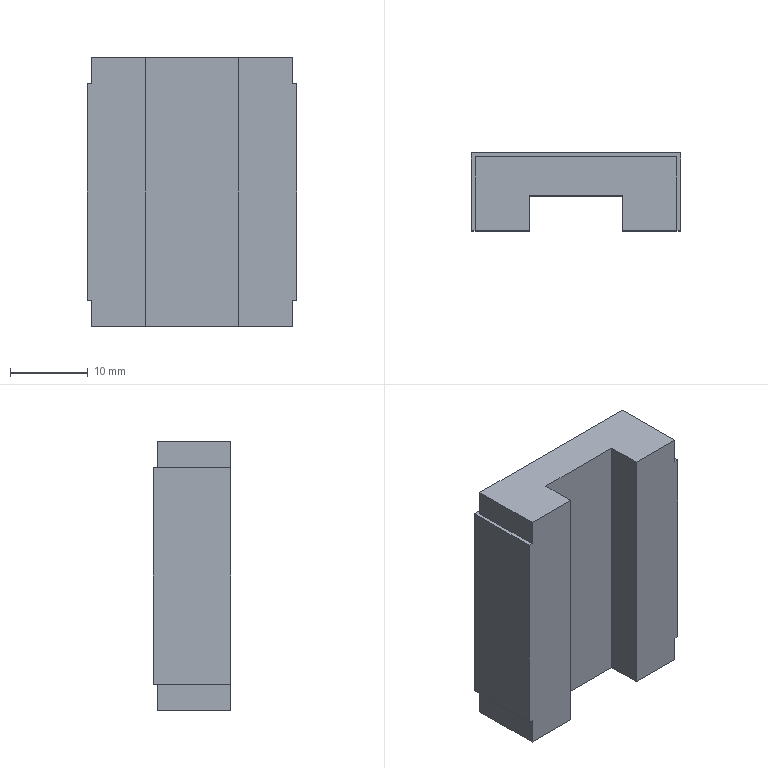Part | NX | features BREP 1 | 1 solid | 34 faces | box 27 x 10 x 34.6 mm | volume 7214 mm3 | plane 18 | cylinder 8 | cone 8 | commonest cylinder face diameters 2.5 x8
STEP:
#1=CARTESIAN_POINT('',(-6.,-0.5,-17.3));
#2=VERTEX_POINT('',#1);
#3=CARTESIAN_POINT('',(6.,-0.5,-17.3));
#4=VERTEX_POINT('',#3);
#5=CARTESIAN_POINT('',(-6.,-0.5,-17.3));
#6=DIRECTION('',(1.,0.,0.));
#7=VECTOR('',#6,1000.);
#8=LINE('',#5,#7);
#9=EDGE_CURVE('',#2,#4,#8,.T.);
#10=ORIENTED_EDGE('',*,*,#9,.T.);
#11=CARTESIAN_POINT('',(6.,-0.5,17.3));
#12=VERTEX_POINT('',#11);
#13=CARTESIAN_POINT('',(6.,-0.5,17.3));
#14=DIRECTION('',(0.,0.,-1.));
#15=VECTOR('',#14,1000.);
#16=LINE('',#13,#15);
#17=EDGE_CURVE('',#12,#4,#16,.T.);
#18=ORIENTED_EDGE('',*,*,#17,.F.);
#19=CARTESIAN_POINT('',(-6.,-0.5,17.3));
#20=VERTEX_POINT('',#19);
#21=CARTESIAN_POINT('',(-6.,-0.5,17.3));
#22=DIRECTION('',(1.,0.,0.));
#23=VECTOR('',#22,1000.);
#24=LINE('',#21,#23);
#25=EDGE_CURVE('',#20,#12,#24,.T.);
#26=ORIENTED_EDGE('',*,*,#25,.F.);
#27=CARTESIAN_POINT('',(-6.,-0.5,17.3));
#28=DIRECTION('',(0.,0.,-1.));
#29=VECTOR('',#28,1000.);
#30=LINE('',#27,#29);
#31=EDGE_CURVE('',#20,#2,#30,.T.);
#32=ORIENTED_EDGE('',*,*,#31,.T.);
#33=EDGE_LOOP('',(#10,#18,#26,#32));
#34=FACE_BOUND('',#33,.T.);
#35=CARTESIAN_POINT('',(-6.,-0.5,17.3));
#36=DIRECTION('',(0.,1.,0.));
#37=DIRECTION('',(-1.,0.,0.));
#38=AXIS2_PLACEMENT_3D('',#35,#36,#37);
#39=PLANE('',#38);
#40=ADVANCED_FACE('',(#34),#39,.F.);
#41=CARTESIAN_POINT('',(-6.,-5.,-17.3));
#42=VERTEX_POINT('',#41);
#43=CARTESIAN_POINT('',(-6.,-9.5,-17.3));
#44=DIRECTION('',(0.,1.,0.));
#45=VECTOR('',#44,1000.);
#46=LINE('',#43,#45);
#47=EDGE_CURVE('',#42,#2,#46,.T.);
#48=ORIENTED_EDGE('',*,*,#47,.T.);
#49=ORIENTED_EDGE('',*,*,#31,.F.);
#50=CARTESIAN_POINT('',(-6.,-5.,17.3));
#51=VERTEX_POINT('',#50);
#52=CARTESIAN_POINT('',(-6.,0.,17.3));
#53=DIRECTION('',(0.,1.,0.));
#54=VECTOR('',#53,1000.);
#55=LINE('',#52,#54);
#56=EDGE_CURVE('',#51,#20,#55,.T.);
#57=ORIENTED_EDGE('',*,*,#56,.F.);
#58=CARTESIAN_POINT('',(-6.,-5.,17.3));
#59=DIRECTION('',(0.,0.,1.));
#60=VECTOR('',#59,1000.);
#61=LINE('',#58,#60);
#62=EDGE_CURVE('',#42,#51,#61,.T.);
#63=ORIENTED_EDGE('',*,*,#62,.F.);
#64=EDGE_LOOP('',(#48,#49,#57,#63));
#65=FACE_BOUND('',#64,.T.);
#66=CARTESIAN_POINT('',(-6.,-9.5,17.3));
#67=DIRECTION('',(-1.,0.,0.));
#68=DIRECTION('',(0.,0.,1.));
#69=AXIS2_PLACEMENT_3D('',#66,#67,#68);
#70=PLANE('',#69);
#71=ADVANCED_FACE('',(#65),#70,.F.);
#72=CARTESIAN_POINT('',(6.,-5.,17.3));
#73=VERTEX_POINT('',#72);
#74=CARTESIAN_POINT('',(6.,-9.5,17.3));
#75=DIRECTION('',(0.,-1.,0.));
#76=VECTOR('',#75,1000.);
#77=LINE('',#74,#76);
#78=EDGE_CURVE('',#12,#73,#77,.T.);
#79=ORIENTED_EDGE('',*,*,#78,.F.);
#80=ORIENTED_EDGE('',*,*,#17,.T.);
#81=CARTESIAN_POINT('',(6.,-5.,-17.3));
#82=VERTEX_POINT('',#81);
#83=CARTESIAN_POINT('',(6.,-9.5,-17.3));
#84=DIRECTION('',(0.,-1.,0.));
#85=VECTOR('',#84,1000.);
#86=LINE('',#83,#85);
#87=EDGE_CURVE('',#4,#82,#86,.T.);
#88=ORIENTED_EDGE('',*,*,#87,.T.);
#89=CARTESIAN_POINT('',(6.,-5.,17.3));
#90=DIRECTION('',(0.,0.,-1.));
#91=VECTOR('',#90,1000.);
#92=LINE('',#89,#91);
#93=EDGE_CURVE('',#73,#82,#92,.T.);
#94=ORIENTED_EDGE('',*,*,#93,.F.);
#95=EDGE_LOOP('',(#79,#80,#88,#94));
#96=FACE_BOUND('',#95,.T.);
#97=CARTESIAN_POINT('',(6.,-9.5,17.3));
#98=DIRECTION('',(1.,0.,0.));
#99=DIRECTION('',(0.,0.,-1.));
#100=AXIS2_PLACEMENT_3D('',#97,#98,#99);
#101=PLANE('',#100);
#102=ADVANCED_FACE('',(#96),#101,.F.);
#103=CARTESIAN_POINT('',(-10.,5.,6.25));
#104=VERTEX_POINT('',#103);
#105=CARTESIAN_POINT('',(-10.,-0.1,6.25));
#106=VERTEX_POINT('',#105);
#107=CARTESIAN_POINT('',(-10.,5.,6.25));
#108=DIRECTION('',(0.,1.,0.));
#109=VECTOR('',#108,1000.);
#110=LINE('',#107,#109);
#111=EDGE_CURVE('',#104,#106,#110,.F.);
#112=ORIENTED_EDGE('',*,*,#111,.T.);
#113=CARTESIAN_POINT('',(-10.,-0.1,8.75));
#114=VERTEX_POINT('',#113);
#115=CARTESIAN_POINT('',(-10.,-0.1,7.5));
#116=DIRECTION('',(0.,1.,0.));
#117=DIRECTION('',(0.,0.,1.));
#118=AXIS2_PLACEMENT_3D('',#115,#116,#117);
#119=CIRCLE('',#118,1.25);
#120=EDGE_CURVE('',#114,#106,#119,.T.);
#121=ORIENTED_EDGE('',*,*,#120,.F.);
#122=CARTESIAN_POINT('',(-10.,5.,8.75));
#123=VERTEX_POINT('',#122);
#124=CARTESIAN_POINT('',(-10.,5.,8.75));
#125=DIRECTION('',(0.,1.,0.));
#126=VECTOR('',#125,1000.);
#127=LINE('',#124,#126);
#128=EDGE_CURVE('',#123,#114,#127,.F.);
#129=ORIENTED_EDGE('',*,*,#128,.F.);
#130=CARTESIAN_POINT('',(-10.,5.,7.5));
#131=DIRECTION('',(0.,1.,0.));
#132=DIRECTION('',(0.,0.,1.));
#133=AXIS2_PLACEMENT_3D('',#130,#131,#132);
#134=CIRCLE('',#133,1.25);
#135=EDGE_CURVE('',#123,#104,#134,.T.);
#136=ORIENTED_EDGE('',*,*,#135,.T.);
#137=EDGE_LOOP('',(#112,#121,#129,#136));
#138=FACE_BOUND('',#137,.T.);
#139=CARTESIAN_POINT('',(-10.,5.,7.5));
#140=DIRECTION('',(0.,1.,0.));
#141=DIRECTION('',(0.,0.,1.));
#142=AXIS2_PLACEMENT_3D('',#139,#140,#141);
#143=CYLINDRICAL_SURFACE('',#142,1.25);
#144=ADVANCED_FACE('',(#138),#143,.F.);
#145=CARTESIAN_POINT('',(-10.,-0.8511,7.5));
#146=VERTEX_POINT('',#145);
#147=CARTESIAN_POINT('',(-10.,-0.1,6.25));
#148=DIRECTION('',(0.,0.515,-0.8572));
#149=VECTOR('',#148,1000.);
#150=LINE('',#147,#149);
#151=EDGE_CURVE('',#146,#106,#150,.T.);
#152=ORIENTED_EDGE('',*,*,#151,.F.);
#153=CARTESIAN_POINT('',(-10.,-0.1,8.75));
#154=DIRECTION('',(0.,0.515,0.8572));
#155=VECTOR('',#154,1000.);
#156=LINE('',#153,#155);
#157=EDGE_CURVE('',#146,#114,#156,.T.);
#158=ORIENTED_EDGE('',*,*,#157,.T.);
#159=ORIENTED_EDGE('',*,*,#120,.T.);
#160=EDGE_LOOP('',(#152,#158,#159));
#161=FACE_BOUND('',#160,.T.);
#162=CARTESIAN_POINT('',(-10.,-0.1,7.5));
#163=DIRECTION('',(0.,1.,0.));
#164=DIRECTION('',(0.,0.,1.));
#165=AXIS2_PLACEMENT_3D('',#162,#163,#164);
#166=CONICAL_SURFACE('',#165,1.25,1.03);
#167=ADVANCED_FACE('',(#161),#166,.F.);
#168=CARTESIAN_POINT('',(10.,5.,6.25));
#169=VERTEX_POINT('',#168);
#170=CARTESIAN_POINT('',(10.,-0.1,6.25));
#171=VERTEX_POINT('',#170);
#172=CARTESIAN_POINT('',(10.,5.,6.25));
#173=DIRECTION('',(0.,1.,0.));
#174=VECTOR('',#173,1000.);
#175=LINE('',#172,#174);
#176=EDGE_CURVE('',#169,#171,#175,.F.);
#177=ORIENTED_EDGE('',*,*,#176,.T.);
#178=CARTESIAN_POINT('',(10.,-0.1,8.75));
#179=VERTEX_POINT('',#178);
#180=CARTESIAN_POINT('',(10.,-0.1,7.5));
#181=DIRECTION('',(0.,1.,0.));
#182=DIRECTION('',(0.,0.,1.));
#183=AXIS2_PLACEMENT_3D('',#180,#181,#182);
#184=CIRCLE('',#183,1.25);
#185=EDGE_CURVE('',#179,#171,#184,.T.);
#186=ORIENTED_EDGE('',*,*,#185,.F.);
#187=CARTESIAN_POINT('',(10.,5.,8.75));
#188=VERTEX_POINT('',#187);
#189=CARTESIAN_POINT('',(10.,5.,8.75));
#190=DIRECTION('',(0.,1.,0.));
#191=VECTOR('',#190,1000.);
#192=LINE('',#189,#191);
#193=EDGE_CURVE('',#188,#179,#192,.F.);
#194=ORIENTED_EDGE('',*,*,#193,.F.);
#195=CARTESIAN_POINT('',(10.,5.,7.5));
#196=DIRECTION('',(0.,1.,0.));
#197=DIRECTION('',(0.,0.,1.));
#198=AXIS2_PLACEMENT_3D('',#195,#196,#197);
#199=CIRCLE('',#198,1.25);
#200=EDGE_CURVE('',#188,#169,#199,.T.);
#201=ORIENTED_EDGE('',*,*,#200,.T.);
#202=EDGE_LOOP('',(#177,#186,#194,#201));
#203=FACE_BOUND('',#202,.T.);
#204=CARTESIAN_POINT('',(10.,5.,7.5));
#205=DIRECTION('',(0.,1.,0.));
#206=DIRECTION('',(0.,0.,1.));
#207=AXIS2_PLACEMENT_3D('',#204,#205,#206);
#208=CYLINDRICAL_SURFACE('',#207,1.25);
#209=ADVANCED_FACE('',(#203),#208,.F.);
#210=CARTESIAN_POINT('',(10.,-0.8511,7.5));
#211=VERTEX_POINT('',#210);
#212=CARTESIAN_POINT('',(10.,-0.1,6.25));
#213=DIRECTION('',(0.,0.515,-0.8572));
#214=VECTOR('',#213,1000.);
#215=LINE('',#212,#214);
#216=EDGE_CURVE('',#211,#171,#215,.T.);
#217=ORIENTED_EDGE('',*,*,#216,.F.);
#218=CARTESIAN_POINT('',(10.,-0.1,8.75));
#219=DIRECTION('',(0.,0.515,0.8572));
#220=VECTOR('',#219,1000.);
#221=LINE('',#218,#220);
#222=EDGE_CURVE('',#211,#179,#221,.T.);
#223=ORIENTED_EDGE('',*,*,#222,.T.);
#224=ORIENTED_EDGE('',*,*,#185,.T.);
#225=EDGE_LOOP('',(#217,#223,#224));
#226=FACE_BOUND('',#225,.T.);
#227=CARTESIAN_POINT('',(10.,-0.1,7.5));
#228=DIRECTION('',(0.,1.,0.));
#229=DIRECTION('',(0.,0.,1.));
#230=AXIS2_PLACEMENT_3D('',#227,#228,#229);
#231=CONICAL_SURFACE('',#230,1.25,1.03);
#232=ADVANCED_FACE('',(#226),#231,.F.);
#233=CARTESIAN_POINT('',(-10.,5.,-8.75));
#234=VERTEX_POINT('',#233);
#235=CARTESIAN_POINT('',(-10.,-0.1,-8.75));
#236=VERTEX_POINT('',#235);
#237=CARTESIAN_POINT('',(-10.,5.,-8.75));
#238=DIRECTION('',(0.,1.,0.));
#239=VECTOR('',#238,1000.);
#240=LINE('',#237,#239);
#241=EDGE_CURVE('',#234,#236,#240,.F.);
#242=ORIENTED_EDGE('',*,*,#241,.T.);
#243=CARTESIAN_POINT('',(-10.,-0.1,-6.25));
#244=VERTEX_POINT('',#243);
#245=CARTESIAN_POINT('',(-10.,-0.1,-7.5));
#246=DIRECTION('',(0.,1.,0.));
#247=DIRECTION('',(0.,0.,1.));
#248=AXIS2_PLACEMENT_3D('',#245,#246,#247);
#249=CIRCLE('',#248,1.25);
#250=EDGE_CURVE('',#244,#236,#249,.T.);
#251=ORIENTED_EDGE('',*,*,#250,.F.);
#252=CARTESIAN_POINT('',(-10.,5.,-6.25));
#253=VERTEX_POINT('',#252);
#254=CARTESIAN_POINT('',(-10.,5.,-6.25));
#255=DIRECTION('',(0.,1.,0.));
#256=VECTOR('',#255,1000.);
#257=LINE('',#254,#256);
#258=EDGE_CURVE('',#253,#244,#257,.F.);
#259=ORIENTED_EDGE('',*,*,#258,.F.);
#260=CARTESIAN_POINT('',(-10.,5.,-7.5));
#261=DIRECTION('',(0.,1.,0.));
#262=DIRECTION('',(0.,0.,1.));
#263=AXIS2_PLACEMENT_3D('',#260,#261,#262);
#264=CIRCLE('',#263,1.25);
#265=EDGE_CURVE('',#253,#234,#264,.T.);
#266=ORIENTED_EDGE('',*,*,#265,.T.);
#267=EDGE_LOOP('',(#242,#251,#259,#266));
#268=FACE_BOUND('',#267,.T.);
#269=CARTESIAN_POINT('',(-10.,5.,-7.5));
#270=DIRECTION('',(0.,1.,0.));
#271=DIRECTION('',(0.,0.,1.));
#272=AXIS2_PLACEMENT_3D('',#269,#270,#271);
#273=CYLINDRICAL_SURFACE('',#272,1.25);
#274=ADVANCED_FACE('',(#268),#273,.F.);
#275=CARTESIAN_POINT('',(-10.,-0.8511,-7.5));
#276=VERTEX_POINT('',#275);
#277=CARTESIAN_POINT('',(-10.,-0.1,-8.75));
#278=DIRECTION('',(0.,0.515,-0.8572));
#279=VECTOR('',#278,1000.);
#280=LINE('',#277,#279);
#281=EDGE_CURVE('',#276,#236,#280,.T.);
#282=ORIENTED_EDGE('',*,*,#281,.F.);
#283=CARTESIAN_POINT('',(-10.,-0.1,-6.25));
#284=DIRECTION('',(0.,0.515,0.8572));
#285=VECTOR('',#284,1000.);
#286=LINE('',#283,#285);
#287=EDGE_CURVE('',#276,#244,#286,.T.);
#288=ORIENTED_EDGE('',*,*,#287,.T.);
#289=ORIENTED_EDGE('',*,*,#250,.T.);
#290=EDGE_LOOP('',(#282,#288,#289));
#291=FACE_BOUND('',#290,.T.);
#292=CARTESIAN_POINT('',(-10.,-0.1,-7.5));
#293=DIRECTION('',(0.,1.,0.));
#294=DIRECTION('',(0.,0.,1.));
#295=AXIS2_PLACEMENT_3D('',#292,#293,#294);
#296=CONICAL_SURFACE('',#295,1.25,1.03);
#297=ADVANCED_FACE('',(#291),#296,.F.);
#298=CARTESIAN_POINT('',(10.,5.,-8.75));
#299=VERTEX_POINT('',#298);
#300=CARTESIAN_POINT('',(10.,-0.1,-8.75));
#301=VERTEX_POINT('',#300);
#302=CARTESIAN_POINT('',(10.,5.,-8.75));
#303=DIRECTION('',(0.,1.,0.));
#304=VECTOR('',#303,1000.);
#305=LINE('',#302,#304);
#306=EDGE_CURVE('',#299,#301,#305,.F.);
#307=ORIENTED_EDGE('',*,*,#306,.T.);
#308=CARTESIAN_POINT('',(10.,-0.1,-6.25));
#309=VERTEX_POINT('',#308);
#310=CARTESIAN_POINT('',(10.,-0.1,-7.5));
#311=DIRECTION('',(0.,1.,0.));
#312=DIRECTION('',(0.,0.,1.));
#313=AXIS2_PLACEMENT_3D('',#310,#311,#312);
#314=CIRCLE('',#313,1.25);
#315=EDGE_CURVE('',#309,#301,#314,.T.);
#316=ORIENTED_EDGE('',*,*,#315,.F.);
#317=CARTESIAN_POINT('',(10.,5.,-6.25));
#318=VERTEX_POINT('',#317);
#319=CARTESIAN_POINT('',(10.,5.,-6.25));
#320=DIRECTION('',(0.,1.,0.));
#321=VECTOR('',#320,1000.);
#322=LINE('',#319,#321);
#323=EDGE_CURVE('',#318,#309,#322,.F.);
#324=ORIENTED_EDGE('',*,*,#323,.F.);
#325=CARTESIAN_POINT('',(10.,5.,-7.5));
#326=DIRECTION('',(0.,1.,0.));
#327=DIRECTION('',(0.,0.,1.));
#328=AXIS2_PLACEMENT_3D('',#325,#326,#327);
#329=CIRCLE('',#328,1.25);
#330=EDGE_CURVE('',#318,#299,#329,.T.);
#331=ORIENTED_EDGE('',*,*,#330,.T.);
#332=EDGE_LOOP('',(#307,#316,#324,#331));
#333=FACE_BOUND('',#332,.T.);
#334=CARTESIAN_POINT('',(10.,5.,-7.5));
#335=DIRECTION('',(0.,1.,0.));
#336=DIRECTION('',(0.,0.,1.));
#337=AXIS2_PLACEMENT_3D('',#334,#335,#336);
#338=CYLINDRICAL_SURFACE('',#337,1.25);
#339=ADVANCED_FACE('',(#333),#338,.F.);
#340=CARTESIAN_POINT('',(10.,-0.8511,-7.5));
#341=VERTEX_POINT('',#340);
#342=CARTESIAN_POINT('',(10.,-0.1,-8.75));
#343=DIRECTION('',(0.,0.515,-0.8572));
#344=VECTOR('',#343,1000.);
#345=LINE('',#342,#344);
#346=EDGE_CURVE('',#341,#301,#345,.T.);
#347=ORIENTED_EDGE('',*,*,#346,.F.);
#348=CARTESIAN_POINT('',(10.,-0.1,-6.25));
#349=DIRECTION('',(0.,0.515,0.8572));
#350=VECTOR('',#349,1000.);
#351=LINE('',#348,#350);
#352=EDGE_CURVE('',#341,#309,#351,.T.);
#353=ORIENTED_EDGE('',*,*,#352,.T.);
#354=ORIENTED_EDGE('',*,*,#315,.T.);
#355=EDGE_LOOP('',(#347,#353,#354));
#356=FACE_BOUND('',#355,.T.);
#357=CARTESIAN_POINT('',(10.,-0.1,-7.5));
#358=DIRECTION('',(0.,1.,0.));
#359=DIRECTION('',(0.,0.,1.));
#360=AXIS2_PLACEMENT_3D('',#357,#358,#359);
#361=CONICAL_SURFACE('',#360,1.25,1.03);
#362=ADVANCED_FACE('',(#356),#361,.F.);
#363=CARTESIAN_POINT('',(13.,4.5,-17.3));
#364=VERTEX_POINT('',#363);
#365=CARTESIAN_POINT('',(13.,-5.,-17.3));
#366=VERTEX_POINT('',#365);
#367=CARTESIAN_POINT('',(13.,4.5,-17.3));
#368=DIRECTION('',(0.,-1.,0.));
#369=VECTOR('',#368,1000.);
#370=LINE('',#367,#369);
#371=EDGE_CURVE('',#364,#366,#370,.T.);
#372=ORIENTED_EDGE('',*,*,#371,.F.);
#373=CARTESIAN_POINT('',(13.,4.5,-13.95));
#374=VERTEX_POINT('',#373);
#375=CARTESIAN_POINT('',(13.,4.5,-13.95));
#376=DIRECTION('',(0.,0.,-1.));
#377=VECTOR('',#376,1000.);
#378=LINE('',#375,#377);
#379=EDGE_CURVE('',#374,#364,#378,.T.);
#380=ORIENTED_EDGE('',*,*,#379,.F.);
#381=CARTESIAN_POINT('',(13.,-5.,-13.95));
#382=VERTEX_POINT('',#381);
#383=CARTESIAN_POINT('',(13.,4.5,-13.95));
#384=DIRECTION('',(0.,-1.,0.));
#385=VECTOR('',#384,1000.);
#386=LINE('',#383,#385);
#387=EDGE_CURVE('',#374,#382,#386,.T.);
#388=ORIENTED_EDGE('',*,*,#387,.T.);
#389=CARTESIAN_POINT('',(13.,-5.,-13.95));
#390=DIRECTION('',(0.,0.,-1.));
#391=VECTOR('',#390,1000.);
#392=LINE('',#389,#391);
#393=EDGE_CURVE('',#382,#366,#392,.T.);
#394=ORIENTED_EDGE('',*,*,#393,.T.);
#395=EDGE_LOOP('',(#372,#380,#388,#394));
#396=FACE_BOUND('',#395,.T.);
#397=CARTESIAN_POINT('',(13.,4.5,-13.95));
#398=DIRECTION('',(1.,0.,0.));
#399=DIRECTION('',(0.,0.,-1.));
#400=AXIS2_PLACEMENT_3D('',#397,#398,#399);
#401=PLANE('',#400);
#402=ADVANCED_FACE('',(#396),#401,.T.);
#403=CARTESIAN_POINT('',(-13.,4.5,-17.3));
#404=VERTEX_POINT('',#403);
#405=CARTESIAN_POINT('',(-13.,4.5,-17.3));
#406=DIRECTION('',(1.,0.,0.));
#407=VECTOR('',#406,1000.);
#408=LINE('',#405,#407);
#409=EDGE_CURVE('',#404,#364,#408,.T.);
#410=ORIENTED_EDGE('',*,*,#409,.F.);
#411=CARTESIAN_POINT('',(-13.,4.5,-13.95));
#412=VERTEX_POINT('',#411);
#413=CARTESIAN_POINT('',(-13.,4.5,-13.95));
#414=DIRECTION('',(0.,0.,-1.));
#415=VECTOR('',#414,1000.);
#416=LINE('',#413,#415);
#417=EDGE_CURVE('',#412,#404,#416,.T.);
#418=ORIENTED_EDGE('',*,*,#417,.F.);
#419=CARTESIAN_POINT('',(-13.,4.5,-13.95));
#420=DIRECTION('',(1.,0.,0.));
#421=VECTOR('',#420,1000.);
#422=LINE('',#419,#421);
#423=EDGE_CURVE('',#412,#374,#422,.T.);
#424=ORIENTED_EDGE('',*,*,#423,.T.);
#425=ORIENTED_EDGE('',*,*,#379,.T.);
#426=EDGE_LOOP('',(#410,#418,#424,#425));
#427=FACE_BOUND('',#426,.T.);
#428=CARTESIAN_POINT('',(-13.,4.5,-13.95));
#429=DIRECTION('',(0.,1.,0.));
#430=DIRECTION('',(-1.,0.,0.));
#431=AXIS2_PLACEMENT_3D('',#428,#429,#430);
#432=PLANE('',#431);
#433=ADVANCED_FACE('',(#427),#432,.T.);
#434=CARTESIAN_POINT('',(-13.,-5.,-17.3));
#435=VERTEX_POINT('',#434);
#436=CARTESIAN_POINT('',(-13.,-5.,-17.3));
#437=DIRECTION('',(0.,1.,0.));
#438=VECTOR('',#437,1000.);
#439=LINE('',#436,#438);
#440=EDGE_CURVE('',#435,#404,#439,.T.);
#441=ORIENTED_EDGE('',*,*,#440,.F.);
#442=CARTESIAN_POINT('',(-13.,-5.,-13.95));
#443=VERTEX_POINT('',#442);
#444=CARTESIAN_POINT('',(-13.,-5.,-13.95));
#445=DIRECTION('',(0.,0.,-1.));
#446=VECTOR('',#445,1000.);
#447=LINE('',#444,#446);
#448=EDGE_CURVE('',#443,#435,#447,.T.);
#449=ORIENTED_EDGE('',*,*,#448,.F.);
#450=CARTESIAN_POINT('',(-13.,-5.,-13.95));
#451=DIRECTION('',(0.,1.,0.));
#452=VECTOR('',#451,1000.);
#453=LINE('',#450,#452);
#454=EDGE_CURVE('',#443,#412,#453,.T.);
#455=ORIENTED_EDGE('',*,*,#454,.T.);
#456=ORIENTED_EDGE('',*,*,#417,.T.);
#457=EDGE_LOOP('',(#441,#449,#455,#456));
#458=FACE_BOUND('',#457,.T.);
#459=CARTESIAN_POINT('',(-13.,-5.,-13.95));
#460=DIRECTION('',(-1.,0.,0.));
#461=DIRECTION('',(0.,0.,1.));
#462=AXIS2_PLACEMENT_3D('',#459,#460,#461);
#463=PLANE('',#462);
#464=ADVANCED_FACE('',(#458),#463,.T.);
#465=CARTESIAN_POINT('',(13.5,5.,-13.95));
#466=VERTEX_POINT('',#465);
#467=CARTESIAN_POINT('',(13.5,-5.,-13.95));
#468=VERTEX_POINT('',#467);
#469=CARTESIAN_POINT('',(13.5,-5.,-13.95));
#470=DIRECTION('',(0.,-1.,0.));
#471=VECTOR('',#470,1000.);
#472=LINE('',#469,#471);
#473=EDGE_CURVE('',#466,#468,#472,.T.);
#474=ORIENTED_EDGE('',*,*,#473,.T.);
#475=CARTESIAN_POINT('',(13.,-5.,-13.95));
#476=DIRECTION('',(1.,0.,0.));
#477=VECTOR('',#476,1000.);
#478=LINE('',#475,#477);
#479=EDGE_CURVE('',#382,#468,#478,.T.);
#480=ORIENTED_EDGE('',*,*,#479,.F.);
#481=ORIENTED_EDGE('',*,*,#387,.F.);
#482=ORIENTED_EDGE('',*,*,#423,.F.);
#483=ORIENTED_EDGE('',*,*,#454,.F.);
#484=CARTESIAN_POINT('',(-13.5,-5.,-13.95));
#485=VERTEX_POINT('',#484);
#486=CARTESIAN_POINT('',(-21.138,-5.,-13.95));
#487=DIRECTION('',(1.,0.,0.));
#488=VECTOR('',#487,1000.);
#489=LINE('',#486,#488);
#490=EDGE_CURVE('',#485,#443,#489,.T.);
#491=ORIENTED_EDGE('',*,*,#490,.F.);
#492=CARTESIAN_POINT('',(-13.5,5.,-13.95));
#493=VERTEX_POINT('',#492);
#494=CARTESIAN_POINT('',(-13.5,-5.,-13.95));
#495=DIRECTION('',(0.,1.,0.));
#496=VECTOR('',#495,1000.);
#497=LINE('',#494,#496);
#498=EDGE_CURVE('',#485,#493,#497,.T.);
#499=ORIENTED_EDGE('',*,*,#498,.T.);
#500=CARTESIAN_POINT('',(-13.5,5.,-13.95));
#501=DIRECTION('',(1.,0.,0.));
#502=VECTOR('',#501,1000.);
#503=LINE('',#500,#502);
#504=EDGE_CURVE('',#493,#466,#503,.T.);
#505=ORIENTED_EDGE('',*,*,#504,.T.);
#506=EDGE_LOOP('',(#474,#480,#481,#482,#483,#491,#499,#505));
#507=FACE_BOUND('',#506,.T.);
#508=CARTESIAN_POINT('',(0.,0.,-13.95));
#509=DIRECTION('',(0.,0.,-1.));
#510=DIRECTION('',(1.,0.,0.));
#511=AXIS2_PLACEMENT_3D('',#508,#509,#510);
#512=PLANE('',#511);
#513=ADVANCED_FACE('',(#507),#512,.T.);
#514=CARTESIAN_POINT('',(-13.,-5.,17.3));
#515=VERTEX_POINT('',#514);
#516=CARTESIAN_POINT('',(-13.,4.5,17.3));
#517=VERTEX_POINT('',#516);
#518=CARTESIAN_POINT('',(-13.,-5.,17.3));
#519=DIRECTION('',(0.,1.,0.));
#520=VECTOR('',#519,1000.);
#521=LINE('',#518,#520);
#522=EDGE_CURVE('',#515,#517,#521,.T.);
#523=ORIENTED_EDGE('',*,*,#522,.T.);
#524=CARTESIAN_POINT('',(-13.,4.5,13.95));
#525=VERTEX_POINT('',#524);
#526=CARTESIAN_POINT('',(-13.,4.5,13.95));
#527=DIRECTION('',(0.,0.,1.));
#528=VECTOR('',#527,1000.);
#529=LINE('',#526,#528);
#530=EDGE_CURVE('',#525,#517,#529,.T.);
#531=ORIENTED_EDGE('',*,*,#530,.F.);
#532=CARTESIAN_POINT('',(-13.,-5.,13.95));
#533=VERTEX_POINT('',#532);
#534=CARTESIAN_POINT('',(-13.,-5.,13.95));
#535=DIRECTION('',(0.,1.,0.));
#536=VECTOR('',#535,1000.);
#537=LINE('',#534,#536);
#538=EDGE_CURVE('',#533,#525,#537,.T.);
#539=ORIENTED_EDGE('',*,*,#538,.F.);
#540=CARTESIAN_POINT('',(-13.,-5.,13.95));
#541=DIRECTION('',(0.,0.,1.));
#542=VECTOR('',#541,1000.);
#543=LINE('',#540,#542);
#544=EDGE_CURVE('',#533,#515,#543,.T.);
#545=ORIENTED_EDGE('',*,*,#544,.T.);
#546=EDGE_LOOP('',(#523,#531,#539,#545));
#547=FACE_BOUND('',#546,.T.);
#548=CARTESIAN_POINT('',(-13.,-5.,13.95));
#549=DIRECTION('',(1.,0.,0.));
#550=DIRECTION('',(0.,0.,-1.));
#551=AXIS2_PLACEMENT_3D('',#548,#549,#550);
#552=PLANE('',#551);
#553=ADVANCED_FACE('',(#547),#552,.F.);
#554=CARTESIAN_POINT('',(13.,4.5,17.3));
#555=VERTEX_POINT('',#554);
#556=CARTESIAN_POINT('',(-13.,4.5,17.3));
#557=DIRECTION('',(1.,0.,0.));
#558=VECTOR('',#557,1000.);
#559=LINE('',#556,#558);
#560=EDGE_CURVE('',#517,#555,#559,.T.);
#561=ORIENTED_EDGE('',*,*,#560,.T.);
#562=CARTESIAN_POINT('',(13.,4.5,13.95));
#563=VERTEX_POINT('',#562);
#564=CARTESIAN_POINT('',(13.,4.5,13.95));
#565=DIRECTION('',(0.,0.,1.));
#566=VECTOR('',#565,1000.);
#567=LINE('',#564,#566);
#568=EDGE_CURVE('',#563,#555,#567,.T.);
#569=ORIENTED_EDGE('',*,*,#568,.F.);
#570=CARTESIAN_POINT('',(-13.,4.5,13.95));
#571=DIRECTION('',(1.,0.,0.));
#572=VECTOR('',#571,1000.);
#573=LINE('',#570,#572);
#574=EDGE_CURVE('',#525,#563,#573,.T.);
#575=ORIENTED_EDGE('',*,*,#574,.F.);
#576=ORIENTED_EDGE('',*,*,#530,.T.);
#577=EDGE_LOOP('',(#561,#569,#575,#576));
#578=FACE_BOUND('',#577,.T.);
#579=CARTESIAN_POINT('',(-13.,4.5,13.95));
#580=DIRECTION('',(0.,-1.,0.));
#581=DIRECTION('',(1.,0.,0.));
#582=AXIS2_PLACEMENT_3D('',#579,#580,#581);
#583=PLANE('',#582);
#584=ADVANCED_FACE('',(#578),#583,.F.);
#585=CARTESIAN_POINT('',(13.,-5.,17.3));
#586=VERTEX_POINT('',#585);
#587=CARTESIAN_POINT('',(13.,4.5,17.3));
#588=DIRECTION('',(0.,-1.,0.));
#589=VECTOR('',#588,1000.);
#590=LINE('',#587,#589);
#591=EDGE_CURVE('',#555,#586,#590,.T.);
#592=ORIENTED_EDGE('',*,*,#591,.T.);
#593=CARTESIAN_POINT('',(13.,-5.,13.95));
#594=VERTEX_POINT('',#593);
#595=CARTESIAN_POINT('',(13.,-5.,13.95));
#596=DIRECTION('',(0.,0.,1.));
#597=VECTOR('',#596,1000.);
#598=LINE('',#595,#597);
#599=EDGE_CURVE('',#594,#586,#598,.T.);
#600=ORIENTED_EDGE('',*,*,#599,.F.);
#601=CARTESIAN_POINT('',(13.,4.5,13.95));
#602=DIRECTION('',(0.,-1.,0.));
#603=VECTOR('',#602,1000.);
#604=LINE('',#601,#603);
#605=EDGE_CURVE('',#563,#594,#604,.T.);
#606=ORIENTED_EDGE('',*,*,#605,.F.);
#607=ORIENTED_EDGE('',*,*,#568,.T.);
#608=EDGE_LOOP('',(#592,#600,#606,#607));
#609=FACE_BOUND('',#608,.T.);
#610=CARTESIAN_POINT('',(13.,4.5,13.95));
#611=DIRECTION('',(-1.,0.,0.));
#612=DIRECTION('',(0.,0.,1.));
#613=AXIS2_PLACEMENT_3D('',#610,#611,#612);
#614=PLANE('',#613);
#615=ADVANCED_FACE('',(#609),#614,.F.);
#616=CARTESIAN_POINT('',(13.5,-5.,13.95));
#617=VERTEX_POINT('',#616);
#618=CARTESIAN_POINT('',(13.5,5.,13.95));
#619=VERTEX_POINT('',#618);
#620=CARTESIAN_POINT('',(13.5,-5.,13.95));
#621=DIRECTION('',(0.,1.,0.));
#622=VECTOR('',#621,1000.);
#623=LINE('',#620,#622);
#624=EDGE_CURVE('',#617,#619,#623,.T.);
#625=ORIENTED_EDGE('',*,*,#624,.T.);
#626=CARTESIAN_POINT('',(-13.5,5.,13.95));
#627=VERTEX_POINT('',#626);
#628=CARTESIAN_POINT('',(-13.5,5.,13.95));
#629=DIRECTION('',(-1.,0.,0.));
#630=VECTOR('',#629,1000.);
#631=LINE('',#628,#630);
#632=EDGE_CURVE('',#619,#627,#631,.T.);
#633=ORIENTED_EDGE('',*,*,#632,.T.);
#634=CARTESIAN_POINT('',(-13.5,-5.,13.95));
#635=VERTEX_POINT('',#634);
#636=CARTESIAN_POINT('',(-13.5,-5.,13.95));
#637=DIRECTION('',(0.,-1.,0.));
#638=VECTOR('',#637,1000.);
#639=LINE('',#636,#638);
#640=EDGE_CURVE('',#627,#635,#639,.T.);
#641=ORIENTED_EDGE('',*,*,#640,.T.);
#642=CARTESIAN_POINT('',(-21.138,-5.,13.95));
#643=DIRECTION('',(1.,0.,0.));
#644=VECTOR('',#643,1000.);
#645=LINE('',#642,#644);
#646=EDGE_CURVE('',#635,#533,#645,.T.);
#647=ORIENTED_EDGE('',*,*,#646,.T.);
#648=ORIENTED_EDGE('',*,*,#538,.T.);
#649=ORIENTED_EDGE('',*,*,#574,.T.);
#650=ORIENTED_EDGE('',*,*,#605,.T.);
#651=CARTESIAN_POINT('',(13.,-5.,13.95));
#652=DIRECTION('',(1.,0.,0.));
#653=VECTOR('',#652,1000.);
#654=LINE('',#651,#653);
#655=EDGE_CURVE('',#594,#617,#654,.T.);
#656=ORIENTED_EDGE('',*,*,#655,.T.);
#657=EDGE_LOOP('',(#625,#633,#641,#647,#648,#649,#650,#656));
#658=FACE_BOUND('',#657,.T.);
#659=CARTESIAN_POINT('',(0.,0.,13.95));
#660=DIRECTION('',(0.,0.,1.));
#661=DIRECTION('',(1.,0.,0.));
#662=AXIS2_PLACEMENT_3D('',#659,#660,#661);
#663=PLANE('',#662);
#664=ADVANCED_FACE('',(#658),#663,.T.);
#665=ORIENTED_EDGE('',*,*,#25,.T.);
#666=ORIENTED_EDGE('',*,*,#78,.T.);
#667=CARTESIAN_POINT('',(-13.5,-5.,17.3));
#668=DIRECTION('',(1.,0.,0.));
#669=VECTOR('',#668,1000.);
#670=LINE('',#667,#669);
#671=EDGE_CURVE('',#73,#586,#670,.T.);
#672=ORIENTED_EDGE('',*,*,#671,.T.);
#673=ORIENTED_EDGE('',*,*,#591,.F.);
#674=ORIENTED_EDGE('',*,*,#560,.F.);
#675=ORIENTED_EDGE('',*,*,#522,.F.);
#676=CARTESIAN_POINT('',(-13.5,-5.,17.3));
#677=DIRECTION('',(1.,0.,0.));
#678=VECTOR('',#677,1000.);
#679=LINE('',#676,#678);
#680=EDGE_CURVE('',#515,#51,#679,.T.);
#681=ORIENTED_EDGE('',*,*,#680,.T.);
#682=ORIENTED_EDGE('',*,*,#56,.T.);
#683=EDGE_LOOP('',(#665,#666,#672,#673,#674,#675,#681,#682));
#684=FACE_BOUND('',#683,.T.);
#685=CARTESIAN_POINT('',(0.,0.,17.3));
#686=DIRECTION('',(0.,0.,-1.));
#687=DIRECTION('',(-1.,0.,0.));
#688=AXIS2_PLACEMENT_3D('',#685,#686,#687);
#689=PLANE('',#688);
#690=ADVANCED_FACE('',(#684),#689,.F.);
#691=ORIENTED_EDGE('',*,*,#87,.F.);
#692=ORIENTED_EDGE('',*,*,#9,.F.);
#693=ORIENTED_EDGE('',*,*,#47,.F.);
#694=CARTESIAN_POINT('',(-13.5,-5.,-17.3));
#695=DIRECTION('',(1.,0.,0.));
#696=VECTOR('',#695,1000.);
#697=LINE('',#694,#696);
#698=EDGE_CURVE('',#435,#42,#697,.T.);
#699=ORIENTED_EDGE('',*,*,#698,.F.);
#700=ORIENTED_EDGE('',*,*,#440,.T.);
#701=ORIENTED_EDGE('',*,*,#409,.T.);
#702=ORIENTED_EDGE('',*,*,#371,.T.);
#703=CARTESIAN_POINT('',(-13.5,-5.,-17.3));
#704=DIRECTION('',(1.,0.,0.));
#705=VECTOR('',#704,1000.);
#706=LINE('',#703,#705);
#707=EDGE_CURVE('',#82,#366,#706,.T.);
#708=ORIENTED_EDGE('',*,*,#707,.F.);
#709=EDGE_LOOP('',(#691,#692,#693,#699,#700,#701,#702,#708));
#710=FACE_BOUND('',#709,.T.);
#711=CARTESIAN_POINT('',(0.,0.,-17.3));
#712=DIRECTION('',(0.,0.,-1.));
#713=DIRECTION('',(-1.,0.,0.));
#714=AXIS2_PLACEMENT_3D('',#711,#712,#713);
#715=PLANE('',#714);
#716=ADVANCED_FACE('',(#710),#715,.T.);
#717=ORIENTED_EDGE('',*,*,#698,.T.);
#718=ORIENTED_EDGE('',*,*,#62,.T.);
#719=ORIENTED_EDGE('',*,*,#680,.F.);
#720=ORIENTED_EDGE('',*,*,#544,.F.);
#721=ORIENTED_EDGE('',*,*,#646,.F.);
#722=CARTESIAN_POINT('',(-13.5,-5.,17.3));
#723=DIRECTION('',(0.,0.,-1.));
#724=VECTOR('',#723,1000.);
#725=LINE('',#722,#724);
#726=EDGE_CURVE('',#635,#485,#725,.T.);
#727=ORIENTED_EDGE('',*,*,#726,.T.);
#728=ORIENTED_EDGE('',*,*,#490,.T.);
#729=ORIENTED_EDGE('',*,*,#448,.T.);
#730=EDGE_LOOP('',(#717,#718,#719,#720,#721,#727,#728,#729));
#731=FACE_BOUND('',#730,.T.);
#732=CARTESIAN_POINT('',(-13.5,-5.,17.3));
#733=DIRECTION('',(0.,1.,0.));
#734=DIRECTION('',(0.,0.,1.));
#735=AXIS2_PLACEMENT_3D('',#732,#733,#734);
#736=PLANE('',#735);
#737=ADVANCED_FACE('',(#731),#736,.F.);
#738=ORIENTED_EDGE('',*,*,#498,.F.);
#739=ORIENTED_EDGE('',*,*,#726,.F.);
#740=ORIENTED_EDGE('',*,*,#640,.F.);
#741=CARTESIAN_POINT('',(-13.5,5.,17.3));
#742=DIRECTION('',(0.,0.,-1.));
#743=VECTOR('',#742,1000.);
#744=LINE('',#741,#743);
#745=EDGE_CURVE('',#627,#493,#744,.T.);
#746=ORIENTED_EDGE('',*,*,#745,.T.);
#747=EDGE_LOOP('',(#738,#739,#740,#746));
#748=FACE_BOUND('',#747,.T.);
#749=CARTESIAN_POINT('',(-13.5,-5.,17.3));
#750=DIRECTION('',(1.,0.,0.));
#751=DIRECTION('',(0.,0.,-1.));
#752=AXIS2_PLACEMENT_3D('',#749,#750,#751);
#753=PLANE('',#752);
#754=ADVANCED_FACE('',(#748),#753,.F.);
#755=ORIENTED_EDGE('',*,*,#504,.F.);
#756=ORIENTED_EDGE('',*,*,#745,.F.);
#757=ORIENTED_EDGE('',*,*,#632,.F.);
#758=CARTESIAN_POINT('',(13.5,5.,17.3));
#759=DIRECTION('',(0.,0.,-1.));
#760=VECTOR('',#759,1000.);
#761=LINE('',#758,#760);
#762=EDGE_CURVE('',#619,#466,#761,.T.);
#763=ORIENTED_EDGE('',*,*,#762,.T.);
#764=EDGE_LOOP('',(#755,#756,#757,#763));
#765=FACE_BOUND('',#764,.T.);
#766=ORIENTED_EDGE('',*,*,#330,.F.);
#767=CARTESIAN_POINT('',(10.,5.,-7.5));
#768=DIRECTION('',(0.,1.,0.));
#769=DIRECTION('',(0.,0.,1.));
#770=AXIS2_PLACEMENT_3D('',#767,#768,#769);
#771=CIRCLE('',#770,1.25);
#772=EDGE_CURVE('',#299,#318,#771,.T.);
#773=ORIENTED_EDGE('',*,*,#772,.F.);
#774=EDGE_LOOP('',(#766,#773));
#775=FACE_BOUND('',#774,.T.);
#776=ORIENTED_EDGE('',*,*,#265,.F.);
#777=CARTESIAN_POINT('',(-10.,5.,-7.5));
#778=DIRECTION('',(0.,1.,0.));
#779=DIRECTION('',(0.,0.,1.));
#780=AXIS2_PLACEMENT_3D('',#777,#778,#779);
#781=CIRCLE('',#780,1.25);
#782=EDGE_CURVE('',#234,#253,#781,.T.);
#783=ORIENTED_EDGE('',*,*,#782,.F.);
#784=EDGE_LOOP('',(#776,#783));
#785=FACE_BOUND('',#784,.T.);
#786=ORIENTED_EDGE('',*,*,#200,.F.);
#787=CARTESIAN_POINT('',(10.,5.,7.5));
#788=DIRECTION('',(0.,1.,0.));
#789=DIRECTION('',(0.,0.,1.));
#790=AXIS2_PLACEMENT_3D('',#787,#788,#789);
#791=CIRCLE('',#790,1.25);
#792=EDGE_CURVE('',#169,#188,#791,.T.);
#793=ORIENTED_EDGE('',*,*,#792,.F.);
#794=EDGE_LOOP('',(#786,#793));
#795=FACE_BOUND('',#794,.T.);
#796=ORIENTED_EDGE('',*,*,#135,.F.);
#797=CARTESIAN_POINT('',(-10.,5.,7.5));
#798=DIRECTION('',(0.,1.,0.));
#799=DIRECTION('',(0.,0.,1.));
#800=AXIS2_PLACEMENT_3D('',#797,#798,#799);
#801=CIRCLE('',#800,1.25);
#802=EDGE_CURVE('',#104,#123,#801,.T.);
#803=ORIENTED_EDGE('',*,*,#802,.F.);
#804=EDGE_LOOP('',(#796,#803));
#805=FACE_BOUND('',#804,.T.);
#806=CARTESIAN_POINT('',(-13.5,5.,17.3));
#807=DIRECTION('',(0.,-1.,0.));
#808=DIRECTION('',(0.,0.,-1.));
#809=AXIS2_PLACEMENT_3D('',#806,#807,#808);
#810=PLANE('',#809);
#811=ADVANCED_FACE('',(#765,#775,#785,#795,#805),#810,.F.);
#812=ORIENTED_EDGE('',*,*,#473,.F.);
#813=ORIENTED_EDGE('',*,*,#762,.F.);
#814=ORIENTED_EDGE('',*,*,#624,.F.);
#815=CARTESIAN_POINT('',(13.5,-5.,17.3));
#816=DIRECTION('',(0.,0.,-1.));
#817=VECTOR('',#816,1000.);
#818=LINE('',#815,#817);
#819=EDGE_CURVE('',#617,#468,#818,.T.);
#820=ORIENTED_EDGE('',*,*,#819,.T.);
#821=EDGE_LOOP('',(#812,#813,#814,#820));
#822=FACE_BOUND('',#821,.T.);
#823=CARTESIAN_POINT('',(13.5,-5.,17.3));
#824=DIRECTION('',(-1.,0.,0.));
#825=DIRECTION('',(0.,0.,1.));
#826=AXIS2_PLACEMENT_3D('',#823,#824,#825);
#827=PLANE('',#826);
#828=ADVANCED_FACE('',(#822),#827,.F.);
#829=ORIENTED_EDGE('',*,*,#671,.F.);
#830=ORIENTED_EDGE('',*,*,#93,.T.);
#831=ORIENTED_EDGE('',*,*,#707,.T.);
#832=ORIENTED_EDGE('',*,*,#393,.F.);
#833=ORIENTED_EDGE('',*,*,#479,.T.);
#834=ORIENTED_EDGE('',*,*,#819,.F.);
#835=ORIENTED_EDGE('',*,*,#655,.F.);
#836=ORIENTED_EDGE('',*,*,#599,.T.);
#837=EDGE_LOOP('',(#829,#830,#831,#832,#833,#834,#835,#836));
#838=FACE_BOUND('',#837,.T.);
#839=CARTESIAN_POINT('',(-13.5,-5.,17.3));
#840=DIRECTION('',(0.,1.,0.));
#841=DIRECTION('',(0.,0.,1.));
#842=AXIS2_PLACEMENT_3D('',#839,#840,#841);
#843=PLANE('',#842);
#844=ADVANCED_FACE('',(#838),#843,.F.);
#845=ORIENTED_EDGE('',*,*,#352,.F.);
#846=ORIENTED_EDGE('',*,*,#346,.T.);
#847=CARTESIAN_POINT('',(10.,-0.1,-7.5));
#848=DIRECTION('',(0.,1.,0.));
#849=DIRECTION('',(0.,0.,1.));
#850=AXIS2_PLACEMENT_3D('',#847,#848,#849);
#851=CIRCLE('',#850,1.25);
#852=EDGE_CURVE('',#301,#309,#851,.T.);
#853=ORIENTED_EDGE('',*,*,#852,.T.);
#854=EDGE_LOOP('',(#845,#846,#853));
#855=FACE_BOUND('',#854,.T.);
#856=CARTESIAN_POINT('',(10.,-0.1,-7.5));
#857=DIRECTION('',(0.,1.,0.));
#858=DIRECTION('',(0.,0.,1.));
#859=AXIS2_PLACEMENT_3D('',#856,#857,#858);
#860=CONICAL_SURFACE('',#859,1.25,1.03);
#861=ADVANCED_FACE('',(#855),#860,.F.);
#862=ORIENTED_EDGE('',*,*,#852,.F.);
#863=ORIENTED_EDGE('',*,*,#306,.F.);
#864=ORIENTED_EDGE('',*,*,#772,.T.);
#865=ORIENTED_EDGE('',*,*,#323,.T.);
#866=EDGE_LOOP('',(#862,#863,#864,#865));
#867=FACE_BOUND('',#866,.T.);
#868=CARTESIAN_POINT('',(10.,5.,-7.5));
#869=DIRECTION('',(0.,1.,0.));
#870=DIRECTION('',(0.,0.,1.));
#871=AXIS2_PLACEMENT_3D('',#868,#869,#870);
#872=CYLINDRICAL_SURFACE('',#871,1.25);
#873=ADVANCED_FACE('',(#867),#872,.F.);
#874=ORIENTED_EDGE('',*,*,#287,.F.);
#875=ORIENTED_EDGE('',*,*,#281,.T.);
#876=CARTESIAN_POINT('',(-10.,-0.1,-7.5));
#877=DIRECTION('',(0.,1.,0.));
#878=DIRECTION('',(0.,0.,1.));
#879=AXIS2_PLACEMENT_3D('',#876,#877,#878);
#880=CIRCLE('',#879,1.25);
#881=EDGE_CURVE('',#236,#244,#880,.T.);
#882=ORIENTED_EDGE('',*,*,#881,.T.);
#883=EDGE_LOOP('',(#874,#875,#882));
#884=FACE_BOUND('',#883,.T.);
#885=CARTESIAN_POINT('',(-10.,-0.1,-7.5));
#886=DIRECTION('',(0.,1.,0.));
#887=DIRECTION('',(0.,0.,1.));
#888=AXIS2_PLACEMENT_3D('',#885,#886,#887);
#889=CONICAL_SURFACE('',#888,1.25,1.03);
#890=ADVANCED_FACE('',(#884),#889,.F.);
#891=ORIENTED_EDGE('',*,*,#881,.F.);
#892=ORIENTED_EDGE('',*,*,#241,.F.);
#893=ORIENTED_EDGE('',*,*,#782,.T.);
#894=ORIENTED_EDGE('',*,*,#258,.T.);
#895=EDGE_LOOP('',(#891,#892,#893,#894));
#896=FACE_BOUND('',#895,.T.);
#897=CARTESIAN_POINT('',(-10.,5.,-7.5));
#898=DIRECTION('',(0.,1.,0.));
#899=DIRECTION('',(0.,0.,1.));
#900=AXIS2_PLACEMENT_3D('',#897,#898,#899);
#901=CYLINDRICAL_SURFACE('',#900,1.25);
#902=ADVANCED_FACE('',(#896),#901,.F.);
#903=ORIENTED_EDGE('',*,*,#222,.F.);
#904=ORIENTED_EDGE('',*,*,#216,.T.);
#905=CARTESIAN_POINT('',(10.,-0.1,7.5));
#906=DIRECTION('',(0.,1.,0.));
#907=DIRECTION('',(0.,0.,1.));
#908=AXIS2_PLACEMENT_3D('',#905,#906,#907);
#909=CIRCLE('',#908,1.25);
#910=EDGE_CURVE('',#171,#179,#909,.T.);
#911=ORIENTED_EDGE('',*,*,#910,.T.);
#912=EDGE_LOOP('',(#903,#904,#911));
#913=FACE_BOUND('',#912,.T.);
#914=CARTESIAN_POINT('',(10.,-0.1,7.5));
#915=DIRECTION('',(0.,1.,0.));
#916=DIRECTION('',(0.,0.,1.));
#917=AXIS2_PLACEMENT_3D('',#914,#915,#916);
#918=CONICAL_SURFACE('',#917,1.25,1.03);
#919=ADVANCED_FACE('',(#913),#918,.F.);
#920=ORIENTED_EDGE('',*,*,#910,.F.);
#921=ORIENTED_EDGE('',*,*,#176,.F.);
#922=ORIENTED_EDGE('',*,*,#792,.T.);
#923=ORIENTED_EDGE('',*,*,#193,.T.);
#924=EDGE_LOOP('',(#920,#921,#922,#923));
#925=FACE_BOUND('',#924,.T.);
#926=CARTESIAN_POINT('',(10.,5.,7.5));
#927=DIRECTION('',(0.,1.,0.));
#928=DIRECTION('',(0.,0.,1.));
#929=AXIS2_PLACEMENT_3D('',#926,#927,#928);
#930=CYLINDRICAL_SURFACE('',#929,1.25);
#931=ADVANCED_FACE('',(#925),#930,.F.);
#932=ORIENTED_EDGE('',*,*,#157,.F.);
#933=ORIENTED_EDGE('',*,*,#151,.T.);
#934=CARTESIAN_POINT('',(-10.,-0.1,7.5));
#935=DIRECTION('',(0.,1.,0.));
#936=DIRECTION('',(0.,0.,1.));
#937=AXIS2_PLACEMENT_3D('',#934,#935,#936);
#938=CIRCLE('',#937,1.25);
#939=EDGE_CURVE('',#106,#114,#938,.T.);
#940=ORIENTED_EDGE('',*,*,#939,.T.);
#941=EDGE_LOOP('',(#932,#933,#940));
#942=FACE_BOUND('',#941,.T.);
#943=CARTESIAN_POINT('',(-10.,-0.1,7.5));
#944=DIRECTION('',(0.,1.,0.));
#945=DIRECTION('',(0.,0.,1.));
#946=AXIS2_PLACEMENT_3D('',#943,#944,#945);
#947=CONICAL_SURFACE('',#946,1.25,1.03);
#948=ADVANCED_FACE('',(#942),#947,.F.);
#949=ORIENTED_EDGE('',*,*,#939,.F.);
#950=ORIENTED_EDGE('',*,*,#111,.F.);
#951=ORIENTED_EDGE('',*,*,#802,.T.);
#952=ORIENTED_EDGE('',*,*,#128,.T.);
#953=EDGE_LOOP('',(#949,#950,#951,#952));
#954=FACE_BOUND('',#953,.T.);
#955=CARTESIAN_POINT('',(-10.,5.,7.5));
#956=DIRECTION('',(0.,1.,0.));
#957=DIRECTION('',(0.,0.,1.));
#958=AXIS2_PLACEMENT_3D('',#955,#956,#957);
#959=CYLINDRICAL_SURFACE('',#958,1.25);
#960=ADVANCED_FACE('',(#954),#959,.F.);
#961=CLOSED_SHELL('',(#40,#71,#102,#144,#167,#209,#232,#274,#297,#339,#362,#402,#433,#464,#513,#553,#584,#615,#664,#690,#716,#737,#754,#811,#828,#844,#861,#873,#890,#902,#919,#931,#948,#960));
#962=MANIFOLD_SOLID_BREP('',#961);
#963=(LENGTH_UNIT()NAMED_UNIT(*)SI_UNIT(.MILLI.,.METRE.));
#964=UNCERTAINTY_MEASURE_WITH_UNIT(LENGTH_MEASURE(0.00001),#963,'','');
#965=(NAMED_UNIT(*)PLANE_ANGLE_UNIT()SI_UNIT($,.RADIAN.));
#966=(NAMED_UNIT(*)SI_UNIT($,.STERADIAN.)SOLID_ANGLE_UNIT());
#967=(GEOMETRIC_REPRESENTATION_CONTEXT(3)GLOBAL_UNCERTAINTY_ASSIGNED_CONTEXT((#964))GLOBAL_UNIT_ASSIGNED_CONTEXT((#963,#965,#966))REPRESENTATION_CONTEXT('',''));
#968=ADVANCED_BREP_SHAPE_REPRESENTATION('',(#962),#967);